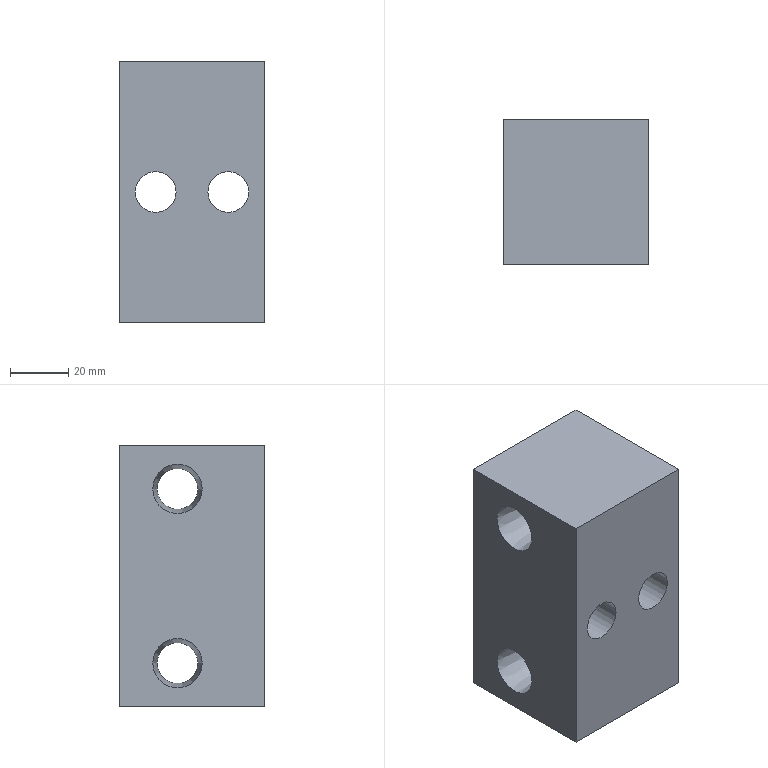Part | NX | features solid 2 | 1 solid | 18 faces | box 50 x 50 x 90 mm | volume 186107 mm3 | plane 8 | cylinder 6 | cone 4 | commonest cylinder face diameters 14 x4 20 x2
STEP:
#1=CARTESIAN_POINT('',(-1485.,-215.,-452.5));
#2=VERTEX_POINT('',#1);
#3=CARTESIAN_POINT('',(-1495.,-215.,-452.5));
#4=DIRECTION('',(0.,-1.,0.));
#5=DIRECTION('',(1.,0.,0.));
#6=AXIS2_PLACEMENT_3D('',#3,#4,#5);
#7=CIRCLE('',#6,10.);
#8=EDGE_CURVE('',#2,#2,#7,.T.);
#9=ORIENTED_EDGE('',*,*,#8,.T.);
#10=EDGE_LOOP('',(#9));
#11=FACE_BOUND('',#10,.T.);
#12=CARTESIAN_POINT('',(-1460.,-215.,-452.5));
#13=VERTEX_POINT('',#12);
#14=CARTESIAN_POINT('',(-1470.,-215.,-452.5));
#15=DIRECTION('',(0.,-1.,0.));
#16=DIRECTION('',(1.,0.,0.));
#17=AXIS2_PLACEMENT_3D('',#14,#15,#16);
#18=CIRCLE('',#17,10.);
#19=EDGE_CURVE('',#13,#13,#18,.T.);
#20=ORIENTED_EDGE('',*,*,#19,.T.);
#21=EDGE_LOOP('',(#20));
#22=FACE_BOUND('',#21,.T.);
#23=CARTESIAN_POINT('',(-1507.5,-215.,-497.5));
#24=VERTEX_POINT('',#23);
#25=CARTESIAN_POINT('',(-1457.5,-215.,-497.5));
#26=VERTEX_POINT('',#25);
#27=CARTESIAN_POINT('',(-1482.5,-215.,-497.5));
#28=DIRECTION('',(1.,0.,0.));
#29=VECTOR('',#28,1000.);
#30=LINE('',#27,#29);
#31=EDGE_CURVE('',#24,#26,#30,.T.);
#32=ORIENTED_EDGE('',*,*,#31,.F.);
#33=CARTESIAN_POINT('',(-1507.5,-215.,-407.5));
#34=VERTEX_POINT('',#33);
#35=CARTESIAN_POINT('',(-1507.5,-215.,-452.5));
#36=DIRECTION('',(0.,0.,-1.));
#37=VECTOR('',#36,1000.);
#38=LINE('',#35,#37);
#39=EDGE_CURVE('',#34,#24,#38,.T.);
#40=ORIENTED_EDGE('',*,*,#39,.F.);
#41=CARTESIAN_POINT('',(-1457.5,-215.,-407.5));
#42=VERTEX_POINT('',#41);
#43=CARTESIAN_POINT('',(-1482.5,-215.,-407.5));
#44=DIRECTION('',(-1.,0.,0.));
#45=VECTOR('',#44,1000.);
#46=LINE('',#43,#45);
#47=EDGE_CURVE('',#42,#34,#46,.T.);
#48=ORIENTED_EDGE('',*,*,#47,.F.);
#49=CARTESIAN_POINT('',(-1457.5,-215.,-452.5));
#50=DIRECTION('',(0.,0.,1.));
#51=VECTOR('',#50,1000.);
#52=LINE('',#49,#51);
#53=EDGE_CURVE('',#26,#42,#52,.T.);
#54=ORIENTED_EDGE('',*,*,#53,.F.);
#55=EDGE_LOOP('',(#32,#40,#48,#54));
#56=FACE_BOUND('',#55,.T.);
#57=CARTESIAN_POINT('',(-1482.5,-215.,-452.5));
#58=DIRECTION('',(0.,1.,0.));
#59=DIRECTION('',(-1.,0.,0.));
#60=AXIS2_PLACEMENT_3D('',#57,#58,#59);
#61=PLANE('',#60);
#62=ADVANCED_FACE('',(#11,#22,#56),#61,.T.);
#63=CARTESIAN_POINT('',(-1507.5,-265.,-497.5));
#64=VERTEX_POINT('',#63);
#65=CARTESIAN_POINT('',(-1507.5,-265.,-497.5));
#66=DIRECTION('',(0.,1.,0.));
#67=VECTOR('',#66,1000.);
#68=LINE('',#65,#67);
#69=EDGE_CURVE('',#64,#24,#68,.T.);
#70=ORIENTED_EDGE('',*,*,#69,.T.);
#71=ORIENTED_EDGE('',*,*,#31,.T.);
#72=CARTESIAN_POINT('',(-1457.5,-265.,-497.5));
#73=VERTEX_POINT('',#72);
#74=CARTESIAN_POINT('',(-1457.5,-265.,-497.5));
#75=DIRECTION('',(0.,1.,0.));
#76=VECTOR('',#75,1000.);
#77=LINE('',#74,#76);
#78=EDGE_CURVE('',#73,#26,#77,.T.);
#79=ORIENTED_EDGE('',*,*,#78,.F.);
#80=CARTESIAN_POINT('',(-1482.5,-265.,-497.5));
#81=DIRECTION('',(-1.,0.,0.));
#82=VECTOR('',#81,1000.);
#83=LINE('',#80,#82);
#84=EDGE_CURVE('',#73,#64,#83,.T.);
#85=ORIENTED_EDGE('',*,*,#84,.T.);
#86=EDGE_LOOP('',(#70,#71,#79,#85));
#87=FACE_BOUND('',#86,.T.);
#88=CARTESIAN_POINT('',(-1482.5,-265.,-497.5));
#89=DIRECTION('',(0.,0.,-1.));
#90=DIRECTION('',(0.,-1.,0.));
#91=AXIS2_PLACEMENT_3D('',#88,#89,#90);
#92=PLANE('',#91);
#93=ADVANCED_FACE('',(#87),#92,.T.);
#94=CARTESIAN_POINT('',(-1457.5,-243.5,-482.5));
#95=VERTEX_POINT('',#94);
#96=CARTESIAN_POINT('',(-1457.5,-235.,-482.5));
#97=DIRECTION('',(-1.,0.,0.));
#98=DIRECTION('',(0.,-1.,0.));
#99=AXIS2_PLACEMENT_3D('',#96,#97,#98);
#100=CIRCLE('',#99,8.5);
#101=EDGE_CURVE('',#95,#95,#100,.T.);
#102=ORIENTED_EDGE('',*,*,#101,.T.);
#103=EDGE_LOOP('',(#102));
#104=FACE_BOUND('',#103,.T.);
#105=CARTESIAN_POINT('',(-1457.5,-243.5,-422.5));
#106=VERTEX_POINT('',#105);
#107=CARTESIAN_POINT('',(-1457.5,-235.,-422.5));
#108=DIRECTION('',(-1.,0.,0.));
#109=DIRECTION('',(0.,-1.,0.));
#110=AXIS2_PLACEMENT_3D('',#107,#108,#109);
#111=CIRCLE('',#110,8.5);
#112=EDGE_CURVE('',#106,#106,#111,.T.);
#113=ORIENTED_EDGE('',*,*,#112,.T.);
#114=EDGE_LOOP('',(#113));
#115=FACE_BOUND('',#114,.T.);
#116=ORIENTED_EDGE('',*,*,#78,.T.);
#117=ORIENTED_EDGE('',*,*,#53,.T.);
#118=CARTESIAN_POINT('',(-1457.5,-265.,-407.5));
#119=VERTEX_POINT('',#118);
#120=CARTESIAN_POINT('',(-1457.5,-265.,-407.5));
#121=DIRECTION('',(0.,1.,0.));
#122=VECTOR('',#121,1000.);
#123=LINE('',#120,#122);
#124=EDGE_CURVE('',#119,#42,#123,.T.);
#125=ORIENTED_EDGE('',*,*,#124,.F.);
#126=CARTESIAN_POINT('',(-1457.5,-265.,-452.5));
#127=DIRECTION('',(0.,0.,-1.));
#128=VECTOR('',#127,1000.);
#129=LINE('',#126,#128);
#130=EDGE_CURVE('',#119,#73,#129,.T.);
#131=ORIENTED_EDGE('',*,*,#130,.T.);
#132=EDGE_LOOP('',(#116,#117,#125,#131));
#133=FACE_BOUND('',#132,.T.);
#134=CARTESIAN_POINT('',(-1457.5,-265.,-452.5));
#135=DIRECTION('',(1.,0.,0.));
#136=DIRECTION('',(0.,1.,0.));
#137=AXIS2_PLACEMENT_3D('',#134,#135,#136);
#138=PLANE('',#137);
#139=ADVANCED_FACE('',(#104,#115,#133),#138,.T.);
#140=ORIENTED_EDGE('',*,*,#124,.T.);
#141=ORIENTED_EDGE('',*,*,#47,.T.);
#142=CARTESIAN_POINT('',(-1507.5,-265.,-407.5));
#143=VERTEX_POINT('',#142);
#144=CARTESIAN_POINT('',(-1507.5,-265.,-407.5));
#145=DIRECTION('',(0.,1.,0.));
#146=VECTOR('',#145,1000.);
#147=LINE('',#144,#146);
#148=EDGE_CURVE('',#143,#34,#147,.T.);
#149=ORIENTED_EDGE('',*,*,#148,.F.);
#150=CARTESIAN_POINT('',(-1482.5,-265.,-407.5));
#151=DIRECTION('',(1.,0.,0.));
#152=VECTOR('',#151,1000.);
#153=LINE('',#150,#152);
#154=EDGE_CURVE('',#143,#119,#153,.T.);
#155=ORIENTED_EDGE('',*,*,#154,.T.);
#156=EDGE_LOOP('',(#140,#141,#149,#155));
#157=FACE_BOUND('',#156,.T.);
#158=CARTESIAN_POINT('',(-1482.5,-265.,-407.5));
#159=DIRECTION('',(0.,0.,1.));
#160=DIRECTION('',(0.,1.,0.));
#161=AXIS2_PLACEMENT_3D('',#158,#159,#160);
#162=PLANE('',#161);
#163=ADVANCED_FACE('',(#157),#162,.T.);
#164=CARTESIAN_POINT('',(-1488.,-265.,-452.5));
#165=VERTEX_POINT('',#164);
#166=CARTESIAN_POINT('',(-1495.,-265.,-452.5));
#167=DIRECTION('',(0.,-1.,0.));
#168=DIRECTION('',(1.,0.,0.));
#169=AXIS2_PLACEMENT_3D('',#166,#167,#168);
#170=CIRCLE('',#169,7.);
#171=EDGE_CURVE('',#165,#165,#170,.T.);
#172=ORIENTED_EDGE('',*,*,#171,.F.);
#173=EDGE_LOOP('',(#172));
#174=FACE_BOUND('',#173,.T.);
#175=CARTESIAN_POINT('',(-1463.,-265.,-452.5));
#176=VERTEX_POINT('',#175);
#177=CARTESIAN_POINT('',(-1470.,-265.,-452.5));
#178=DIRECTION('',(0.,-1.,0.));
#179=DIRECTION('',(1.,0.,0.));
#180=AXIS2_PLACEMENT_3D('',#177,#178,#179);
#181=CIRCLE('',#180,7.);
#182=EDGE_CURVE('',#176,#176,#181,.T.);
#183=ORIENTED_EDGE('',*,*,#182,.F.);
#184=EDGE_LOOP('',(#183));
#185=FACE_BOUND('',#184,.T.);
#186=CARTESIAN_POINT('',(-1507.5,-265.,-452.5));
#187=DIRECTION('',(0.,0.,1.));
#188=VECTOR('',#187,1000.);
#189=LINE('',#186,#188);
#190=EDGE_CURVE('',#64,#143,#189,.T.);
#191=ORIENTED_EDGE('',*,*,#190,.F.);
#192=ORIENTED_EDGE('',*,*,#84,.F.);
#193=ORIENTED_EDGE('',*,*,#130,.F.);
#194=ORIENTED_EDGE('',*,*,#154,.F.);
#195=EDGE_LOOP('',(#191,#192,#193,#194));
#196=FACE_BOUND('',#195,.T.);
#197=CARTESIAN_POINT('',(-1482.5,-265.,-452.5));
#198=DIRECTION('',(0.,-1.,0.));
#199=DIRECTION('',(1.,0.,0.));
#200=AXIS2_PLACEMENT_3D('',#197,#198,#199);
#201=PLANE('',#200);
#202=ADVANCED_FACE('',(#174,#185,#196),#201,.T.);
#203=CARTESIAN_POINT('',(-1507.5,-243.5,-422.5));
#204=VERTEX_POINT('',#203);
#205=CARTESIAN_POINT('',(-1507.5,-235.,-422.5));
#206=DIRECTION('',(-1.,0.,0.));
#207=DIRECTION('',(0.,-1.,0.));
#208=AXIS2_PLACEMENT_3D('',#205,#206,#207);
#209=CIRCLE('',#208,8.5);
#210=EDGE_CURVE('',#204,#204,#209,.T.);
#211=ORIENTED_EDGE('',*,*,#210,.F.);
#212=EDGE_LOOP('',(#211));
#213=FACE_BOUND('',#212,.T.);
#214=CARTESIAN_POINT('',(-1507.5,-243.5,-482.5));
#215=VERTEX_POINT('',#214);
#216=CARTESIAN_POINT('',(-1507.5,-235.,-482.5));
#217=DIRECTION('',(-1.,0.,0.));
#218=DIRECTION('',(0.,-1.,0.));
#219=AXIS2_PLACEMENT_3D('',#216,#217,#218);
#220=CIRCLE('',#219,8.5);
#221=EDGE_CURVE('',#215,#215,#220,.T.);
#222=ORIENTED_EDGE('',*,*,#221,.F.);
#223=EDGE_LOOP('',(#222));
#224=FACE_BOUND('',#223,.T.);
#225=ORIENTED_EDGE('',*,*,#190,.T.);
#226=ORIENTED_EDGE('',*,*,#148,.T.);
#227=ORIENTED_EDGE('',*,*,#39,.T.);
#228=ORIENTED_EDGE('',*,*,#69,.F.);
#229=EDGE_LOOP('',(#225,#226,#227,#228));
#230=FACE_BOUND('',#229,.T.);
#231=CARTESIAN_POINT('',(-1507.5,-265.,-452.5));
#232=DIRECTION('',(-1.,0.,0.));
#233=DIRECTION('',(0.,-1.,0.));
#234=AXIS2_PLACEMENT_3D('',#231,#232,#233);
#235=PLANE('',#234);
#236=ADVANCED_FACE('',(#213,#224,#230),#235,.T.);
#237=ORIENTED_EDGE('',*,*,#182,.T.);
#238=EDGE_LOOP('',(#237));
#239=FACE_BOUND('',#238,.T.);
#240=CARTESIAN_POINT('',(-1463.,-235.,-452.5));
#241=VERTEX_POINT('',#240);
#242=CARTESIAN_POINT('',(-1470.,-235.,-452.5));
#243=DIRECTION('',(0.,-1.,0.));
#244=DIRECTION('',(1.,0.,0.));
#245=AXIS2_PLACEMENT_3D('',#242,#243,#244);
#246=CIRCLE('',#245,7.);
#247=EDGE_CURVE('',#241,#241,#246,.T.);
#248=ORIENTED_EDGE('',*,*,#247,.F.);
#249=EDGE_LOOP('',(#248));
#250=FACE_BOUND('',#249,.T.);
#251=CARTESIAN_POINT('',(-1470.,-315.,-452.5));
#252=DIRECTION('',(0.,-1.,0.));
#253=DIRECTION('',(1.,0.,0.));
#254=AXIS2_PLACEMENT_3D('',#251,#252,#253);
#255=CYLINDRICAL_SURFACE('',#254,7.);
#256=ADVANCED_FACE('',(#239,#250),#255,.F.);
#257=ORIENTED_EDGE('',*,*,#247,.T.);
#258=EDGE_LOOP('',(#257));
#259=FACE_BOUND('',#258,.T.);
#260=CARTESIAN_POINT('',(-1460.,-235.,-452.5));
#261=VERTEX_POINT('',#260);
#262=CARTESIAN_POINT('',(-1470.,-235.,-452.5));
#263=DIRECTION('',(0.,-1.,0.));
#264=DIRECTION('',(1.,0.,0.));
#265=AXIS2_PLACEMENT_3D('',#262,#263,#264);
#266=CIRCLE('',#265,10.);
#267=EDGE_CURVE('',#261,#261,#266,.T.);
#268=ORIENTED_EDGE('',*,*,#267,.F.);
#269=EDGE_LOOP('',(#268));
#270=FACE_BOUND('',#269,.T.);
#271=CARTESIAN_POINT('',(-1470.,-235.,-452.5));
#272=DIRECTION('',(0.,-1.,0.));
#273=DIRECTION('',(1.,0.,0.));
#274=AXIS2_PLACEMENT_3D('',#271,#272,#273);
#275=PLANE('',#274);
#276=ADVANCED_FACE('',(#259,#270),#275,.F.);
#277=ORIENTED_EDGE('',*,*,#267,.T.);
#278=EDGE_LOOP('',(#277));
#279=FACE_BOUND('',#278,.T.);
#280=ORIENTED_EDGE('',*,*,#19,.F.);
#281=EDGE_LOOP('',(#280));
#282=FACE_BOUND('',#281,.T.);
#283=CARTESIAN_POINT('',(-1470.,-215.,-452.5));
#284=DIRECTION('',(0.,-1.,0.));
#285=DIRECTION('',(1.,0.,0.));
#286=AXIS2_PLACEMENT_3D('',#283,#284,#285);
#287=CYLINDRICAL_SURFACE('',#286,10.);
#288=ADVANCED_FACE('',(#279,#282),#287,.F.);
#289=ORIENTED_EDGE('',*,*,#171,.T.);
#290=EDGE_LOOP('',(#289));
#291=FACE_BOUND('',#290,.T.);
#292=CARTESIAN_POINT('',(-1488.,-235.,-452.5));
#293=VERTEX_POINT('',#292);
#294=CARTESIAN_POINT('',(-1495.,-235.,-452.5));
#295=DIRECTION('',(0.,-1.,0.));
#296=DIRECTION('',(1.,0.,0.));
#297=AXIS2_PLACEMENT_3D('',#294,#295,#296);
#298=CIRCLE('',#297,7.);
#299=EDGE_CURVE('',#293,#293,#298,.T.);
#300=ORIENTED_EDGE('',*,*,#299,.F.);
#301=EDGE_LOOP('',(#300));
#302=FACE_BOUND('',#301,.T.);
#303=CARTESIAN_POINT('',(-1495.,-315.,-452.5));
#304=DIRECTION('',(0.,-1.,0.));
#305=DIRECTION('',(1.,0.,0.));
#306=AXIS2_PLACEMENT_3D('',#303,#304,#305);
#307=CYLINDRICAL_SURFACE('',#306,7.);
#308=ADVANCED_FACE('',(#291,#302),#307,.F.);
#309=ORIENTED_EDGE('',*,*,#299,.T.);
#310=EDGE_LOOP('',(#309));
#311=FACE_BOUND('',#310,.T.);
#312=CARTESIAN_POINT('',(-1485.,-235.,-452.5));
#313=VERTEX_POINT('',#312);
#314=CARTESIAN_POINT('',(-1495.,-235.,-452.5));
#315=DIRECTION('',(0.,-1.,0.));
#316=DIRECTION('',(1.,0.,0.));
#317=AXIS2_PLACEMENT_3D('',#314,#315,#316);
#318=CIRCLE('',#317,10.);
#319=EDGE_CURVE('',#313,#313,#318,.T.);
#320=ORIENTED_EDGE('',*,*,#319,.F.);
#321=EDGE_LOOP('',(#320));
#322=FACE_BOUND('',#321,.T.);
#323=CARTESIAN_POINT('',(-1495.,-235.,-452.5));
#324=DIRECTION('',(0.,-1.,0.));
#325=DIRECTION('',(1.,0.,0.));
#326=AXIS2_PLACEMENT_3D('',#323,#324,#325);
#327=PLANE('',#326);
#328=ADVANCED_FACE('',(#311,#322),#327,.F.);
#329=ORIENTED_EDGE('',*,*,#319,.T.);
#330=EDGE_LOOP('',(#329));
#331=FACE_BOUND('',#330,.T.);
#332=ORIENTED_EDGE('',*,*,#8,.F.);
#333=EDGE_LOOP('',(#332));
#334=FACE_BOUND('',#333,.T.);
#335=CARTESIAN_POINT('',(-1495.,-215.,-452.5));
#336=DIRECTION('',(0.,-1.,0.));
#337=DIRECTION('',(1.,0.,0.));
#338=AXIS2_PLACEMENT_3D('',#335,#336,#337);
#339=CYLINDRICAL_SURFACE('',#338,10.);
#340=ADVANCED_FACE('',(#331,#334),#339,.F.);
#341=CARTESIAN_POINT('',(-1469.5,-228.,-482.5));
#342=VERTEX_POINT('',#341);
#343=CARTESIAN_POINT('',(-1469.5,-235.,-482.5));
#344=DIRECTION('',(1.,0.,0.));
#345=DIRECTION('',(0.,1.,0.));
#346=AXIS2_PLACEMENT_3D('',#343,#344,#345);
#347=CIRCLE('',#346,7.);
#348=EDGE_CURVE('',#342,#342,#347,.T.);
#349=ORIENTED_EDGE('',*,*,#348,.T.);
#350=EDGE_LOOP('',(#349));
#351=FACE_BOUND('',#350,.T.);
#352=CARTESIAN_POINT('',(-1495.5,-228.,-482.5));
#353=VERTEX_POINT('',#352);
#354=CARTESIAN_POINT('',(-1495.5,-235.,-482.5));
#355=DIRECTION('',(1.,0.,0.));
#356=DIRECTION('',(0.,1.,0.));
#357=AXIS2_PLACEMENT_3D('',#354,#355,#356);
#358=CIRCLE('',#357,7.);
#359=EDGE_CURVE('',#353,#353,#358,.T.);
#360=ORIENTED_EDGE('',*,*,#359,.F.);
#361=EDGE_LOOP('',(#360));
#362=FACE_BOUND('',#361,.T.);
#363=CARTESIAN_POINT('',(-1507.5,-235.,-482.5));
#364=DIRECTION('',(1.,0.,0.));
#365=DIRECTION('',(0.,1.,0.));
#366=AXIS2_PLACEMENT_3D('',#363,#364,#365);
#367=CYLINDRICAL_SURFACE('',#366,7.);
#368=ADVANCED_FACE('',(#351,#362),#367,.F.);
#369=CARTESIAN_POINT('',(-1469.5,-228.,-422.5));
#370=VERTEX_POINT('',#369);
#371=CARTESIAN_POINT('',(-1469.5,-235.,-422.5));
#372=DIRECTION('',(1.,0.,0.));
#373=DIRECTION('',(0.,1.,0.));
#374=AXIS2_PLACEMENT_3D('',#371,#372,#373);
#375=CIRCLE('',#374,7.);
#376=EDGE_CURVE('',#370,#370,#375,.T.);
#377=ORIENTED_EDGE('',*,*,#376,.T.);
#378=EDGE_LOOP('',(#377));
#379=FACE_BOUND('',#378,.T.);
#380=CARTESIAN_POINT('',(-1495.5,-228.,-422.5));
#381=VERTEX_POINT('',#380);
#382=CARTESIAN_POINT('',(-1495.5,-235.,-422.5));
#383=DIRECTION('',(1.,0.,0.));
#384=DIRECTION('',(0.,1.,0.));
#385=AXIS2_PLACEMENT_3D('',#382,#383,#384);
#386=CIRCLE('',#385,7.);
#387=EDGE_CURVE('',#381,#381,#386,.T.);
#388=ORIENTED_EDGE('',*,*,#387,.F.);
#389=EDGE_LOOP('',(#388));
#390=FACE_BOUND('',#389,.T.);
#391=CARTESIAN_POINT('',(-1507.5,-235.,-422.5));
#392=DIRECTION('',(1.,0.,0.));
#393=DIRECTION('',(0.,1.,0.));
#394=AXIS2_PLACEMENT_3D('',#391,#392,#393);
#395=CYLINDRICAL_SURFACE('',#394,7.);
#396=ADVANCED_FACE('',(#379,#390),#395,.F.);
#397=ORIENTED_EDGE('',*,*,#221,.T.);
#398=EDGE_LOOP('',(#397));
#399=FACE_BOUND('',#398,.T.);
#400=ORIENTED_EDGE('',*,*,#359,.T.);
#401=EDGE_LOOP('',(#400));
#402=FACE_BOUND('',#401,.T.);
#403=CARTESIAN_POINT('',(-1495.5,-235.,-482.5));
#404=DIRECTION('',(-1.,0.,0.));
#405=DIRECTION('',(0.,1.,0.));
#406=AXIS2_PLACEMENT_3D('',#403,#404,#405);
#407=CONICAL_SURFACE('',#406,7.,0.1244);
#408=ADVANCED_FACE('',(#399,#402),#407,.F.);
#409=ORIENTED_EDGE('',*,*,#210,.T.);
#410=EDGE_LOOP('',(#409));
#411=FACE_BOUND('',#410,.T.);
#412=ORIENTED_EDGE('',*,*,#387,.T.);
#413=EDGE_LOOP('',(#412));
#414=FACE_BOUND('',#413,.T.);
#415=CARTESIAN_POINT('',(-1495.5,-235.,-422.5));
#416=DIRECTION('',(-1.,0.,0.));
#417=DIRECTION('',(0.,1.,0.));
#418=AXIS2_PLACEMENT_3D('',#415,#416,#417);
#419=CONICAL_SURFACE('',#418,7.,0.1244);
#420=ADVANCED_FACE('',(#411,#414),#419,.F.);
#421=ORIENTED_EDGE('',*,*,#112,.F.);
#422=EDGE_LOOP('',(#421));
#423=FACE_BOUND('',#422,.T.);
#424=ORIENTED_EDGE('',*,*,#376,.F.);
#425=EDGE_LOOP('',(#424));
#426=FACE_BOUND('',#425,.T.);
#427=CARTESIAN_POINT('',(-1469.5,-235.,-422.5));
#428=DIRECTION('',(1.,0.,0.));
#429=DIRECTION('',(0.,1.,0.));
#430=AXIS2_PLACEMENT_3D('',#427,#428,#429);
#431=CONICAL_SURFACE('',#430,7.,0.1244);
#432=ADVANCED_FACE('',(#423,#426),#431,.F.);
#433=ORIENTED_EDGE('',*,*,#101,.F.);
#434=EDGE_LOOP('',(#433));
#435=FACE_BOUND('',#434,.T.);
#436=ORIENTED_EDGE('',*,*,#348,.F.);
#437=EDGE_LOOP('',(#436));
#438=FACE_BOUND('',#437,.T.);
#439=CARTESIAN_POINT('',(-1469.5,-235.,-482.5));
#440=DIRECTION('',(1.,0.,0.));
#441=DIRECTION('',(0.,1.,0.));
#442=AXIS2_PLACEMENT_3D('',#439,#440,#441);
#443=CONICAL_SURFACE('',#442,7.,0.1244);
#444=ADVANCED_FACE('',(#435,#438),#443,.F.);
#445=CLOSED_SHELL('',(#62,#93,#139,#163,#202,#236,#256,#276,#288,#308,#328,#340,#368,#396,#408,#420,#432,#444));
#446=MANIFOLD_SOLID_BREP('',#445);
#447=(LENGTH_UNIT()NAMED_UNIT(*)SI_UNIT(.MILLI.,.METRE.));
#448=UNCERTAINTY_MEASURE_WITH_UNIT(LENGTH_MEASURE(0.00001),#447,'','');
#449=(NAMED_UNIT(*)PLANE_ANGLE_UNIT()SI_UNIT($,.RADIAN.));
#450=(NAMED_UNIT(*)SI_UNIT($,.STERADIAN.)SOLID_ANGLE_UNIT());
#451=(GEOMETRIC_REPRESENTATION_CONTEXT(3)GLOBAL_UNCERTAINTY_ASSIGNED_CONTEXT((#448))GLOBAL_UNIT_ASSIGNED_CONTEXT((#447,#449,#450))REPRESENTATION_CONTEXT('',''));
#452=ADVANCED_BREP_SHAPE_REPRESENTATION('',(#446),#451);